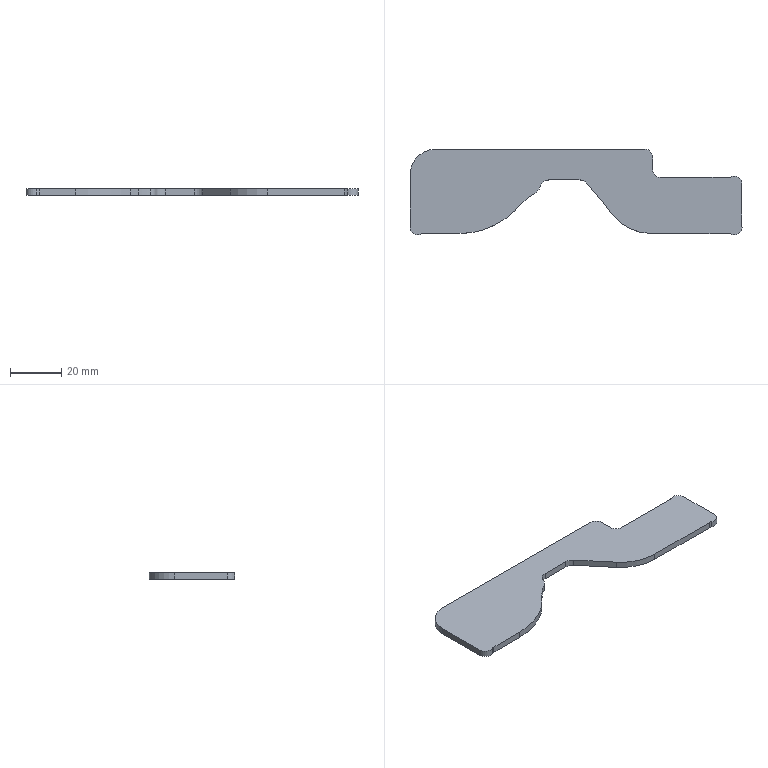Part | STEP file | lll_id342_x_t | 1 solid | 27 faces | box 130 x 33.5 x 2.5 mm | volume 7847 mm3 | cylinder 15 | plane 12 | commonest cylinder face diameters 6 x8 8 x3 20 x1 38 x1 39.772 x1 59.996 x1
STEP:
#1=CARTESIAN_POINT('',(708.5,-40.5,0.));
#2=VERTEX_POINT('',#1);
#3=CARTESIAN_POINT('',(708.5,-40.5,2.5));
#4=VERTEX_POINT('',#3);
#5=CARTESIAN_POINT('',(708.5,-40.5,-2.5));
#6=DIRECTION('',(0.,0.,1.));
#7=VECTOR('',#6,1.);
#8=LINE('',#5,#7);
#9=EDGE_CURVE('',#2,#4,#8,.T.);
#10=ORIENTED_EDGE('',*,*,#9,.T.);
#11=CARTESIAN_POINT('',(693.945,-33.713,2.5));
#12=VERTEX_POINT('',#11);
#13=CARTESIAN_POINT('',(708.5,-21.5,2.5));
#14=DIRECTION('',(0.,0.,-1.));
#15=DIRECTION('',(-1.,0.,0.));
#16=AXIS2_PLACEMENT_3D('',#13,#14,#15);
#17=CIRCLE('',#16,19.);
#18=EDGE_CURVE('',#4,#12,#17,.T.);
#19=ORIENTED_EDGE('',*,*,#18,.T.);
#20=CARTESIAN_POINT('',(693.945,-33.713,0.));
#21=VERTEX_POINT('',#20);
#22=CARTESIAN_POINT('',(693.945,-33.713,-2.5));
#23=DIRECTION('',(0.,0.,1.));
#24=VECTOR('',#23,1.);
#25=LINE('',#22,#24);
#26=EDGE_CURVE('',#21,#12,#25,.T.);
#27=ORIENTED_EDGE('',*,*,#26,.F.);
#28=CARTESIAN_POINT('',(708.5,-21.5,0.));
#29=DIRECTION('',(0.,0.,1.));
#30=DIRECTION('',(-1.,0.,0.));
#31=AXIS2_PLACEMENT_3D('',#28,#29,#30);
#32=CIRCLE('',#31,19.);
#33=EDGE_CURVE('',#21,#2,#32,.T.);
#34=ORIENTED_EDGE('',*,*,#33,.T.);
#35=EDGE_LOOP('',(#10,#19,#27,#34));
#36=FACE_OUTER_BOUND('',#35,.T.);
#37=CARTESIAN_POINT('',(708.5,-21.5,-2.5));
#38=DIRECTION('',(0.,0.,1.));
#39=DIRECTION('',(1.,0.,0.));
#40=AXIS2_PLACEMENT_3D('',#37,#38,#39);
#41=CYLINDRICAL_SURFACE('',#40,19.);
#42=ADVANCED_FACE('',(#36),#41,.T.);
#43=CARTESIAN_POINT('',(738.602,-40.5,0.));
#44=VERTEX_POINT('',#43);
#45=CARTESIAN_POINT('',(738.602,-40.5,2.5));
#46=VERTEX_POINT('',#45);
#47=CARTESIAN_POINT('',(738.602,-40.5,-2.5));
#48=DIRECTION('',(0.,0.,1.));
#49=VECTOR('',#48,1.);
#50=LINE('',#47,#49);
#51=EDGE_CURVE('',#44,#46,#50,.T.);
#52=ORIENTED_EDGE('',*,*,#51,.T.);
#53=CARTESIAN_POINT('',(12273.883,-40.5,2.5));
#54=DIRECTION('',(-1.,0.,0.));
#55=VECTOR('',#54,1.);
#56=LINE('',#53,#55);
#57=EDGE_CURVE('',#46,#4,#56,.T.);
#58=ORIENTED_EDGE('',*,*,#57,.T.);
#59=ORIENTED_EDGE('',*,*,#9,.F.);
#60=CARTESIAN_POINT('',(12283.883,-40.5,0.));
#61=DIRECTION('',(-1.,0.,0.));
#62=VECTOR('',#61,1.);
#63=LINE('',#60,#62);
#64=EDGE_CURVE('',#44,#2,#63,.T.);
#65=ORIENTED_EDGE('',*,*,#64,.F.);
#66=EDGE_LOOP('',(#52,#58,#59,#65));
#67=FACE_OUTER_BOUND('',#66,.T.);
#68=CARTESIAN_POINT('',(708.5,-40.5,-2.5));
#69=DIRECTION('',(0.,-1.,0.));
#70=DIRECTION('',(1.,0.,0.));
#71=AXIS2_PLACEMENT_3D('',#68,#69,#70);
#72=PLANE('',#71);
#73=ADVANCED_FACE('',(#67),#72,.T.);
#74=CARTESIAN_POINT('',(739.801,-40.75,0.));
#75=VERTEX_POINT('',#74);
#76=CARTESIAN_POINT('',(739.801,-40.75,2.5));
#77=VERTEX_POINT('',#76);
#78=CARTESIAN_POINT('',(739.801,-40.75,-2.5));
#79=DIRECTION('',(0.,0.,1.));
#80=VECTOR('',#79,1.);
#81=LINE('',#78,#80);
#82=EDGE_CURVE('',#75,#77,#81,.T.);
#83=ORIENTED_EDGE('',*,*,#82,.T.);
#84=CARTESIAN_POINT('',(738.602,-43.5,2.5));
#85=DIRECTION('',(0.,0.,1.));
#86=DIRECTION('',(-1.,0.,0.));
#87=AXIS2_PLACEMENT_3D('',#84,#85,#86);
#88=CIRCLE('',#87,3.);
#89=EDGE_CURVE('',#77,#46,#88,.T.);
#90=ORIENTED_EDGE('',*,*,#89,.T.);
#91=ORIENTED_EDGE('',*,*,#51,.F.);
#92=CARTESIAN_POINT('',(738.602,-43.5,0.));
#93=DIRECTION('',(0.,0.,-1.));
#94=DIRECTION('',(-1.,0.,0.));
#95=AXIS2_PLACEMENT_3D('',#92,#93,#94);
#96=CIRCLE('',#95,3.);
#97=EDGE_CURVE('',#44,#75,#96,.T.);
#98=ORIENTED_EDGE('',*,*,#97,.T.);
#99=EDGE_LOOP('',(#83,#90,#91,#98));
#100=FACE_OUTER_BOUND('',#99,.T.);
#101=CARTESIAN_POINT('',(738.602,-43.5,-2.5));
#102=DIRECTION('',(0.,0.,1.));
#103=DIRECTION('',(1.,0.,0.));
#104=AXIS2_PLACEMENT_3D('',#101,#102,#103);
#105=CYLINDRICAL_SURFACE('',#104,3.);
#106=ADVANCED_FACE('',(#100),#105,.F.);
#107=CARTESIAN_POINT('',(744.,-38.,0.));
#108=VERTEX_POINT('',#107);
#109=CARTESIAN_POINT('',(744.,-38.,2.5));
#110=VERTEX_POINT('',#109);
#111=CARTESIAN_POINT('',(744.,-38.,-2.5));
#112=DIRECTION('',(0.,0.,1.));
#113=VECTOR('',#112,1.);
#114=LINE('',#111,#113);
#115=EDGE_CURVE('',#108,#110,#114,.T.);
#116=ORIENTED_EDGE('',*,*,#115,.T.);
#117=CARTESIAN_POINT('',(741.,-38.,2.5));
#118=DIRECTION('',(0.,0.,-1.));
#119=DIRECTION('',(-1.,0.,0.));
#120=AXIS2_PLACEMENT_3D('',#117,#118,#119);
#121=CIRCLE('',#120,3.);
#122=EDGE_CURVE('',#110,#77,#121,.T.);
#123=ORIENTED_EDGE('',*,*,#122,.T.);
#124=ORIENTED_EDGE('',*,*,#82,.F.);
#125=CARTESIAN_POINT('',(741.,-38.,0.));
#126=DIRECTION('',(0.,0.,-1.));
#127=DIRECTION('',(-1.,0.,0.));
#128=AXIS2_PLACEMENT_3D('',#125,#126,#127);
#129=CIRCLE('',#128,3.);
#130=EDGE_CURVE('',#108,#75,#129,.T.);
#131=ORIENTED_EDGE('',*,*,#130,.F.);
#132=EDGE_LOOP('',(#116,#123,#124,#131));
#133=FACE_OUTER_BOUND('',#132,.T.);
#134=CARTESIAN_POINT('',(741.,-38.,-2.5));
#135=DIRECTION('',(0.,0.,1.));
#136=DIRECTION('',(1.,0.,0.));
#137=AXIS2_PLACEMENT_3D('',#134,#135,#136);
#138=CYLINDRICAL_SURFACE('',#137,3.);
#139=ADVANCED_FACE('',(#133),#138,.T.);
#140=ORIENTED_EDGE('',*,*,#26,.T.);
#141=CARTESIAN_POINT('',(683.218,-20.929,2.5));
#142=VERTEX_POINT('',#141);
#143=CARTESIAN_POINT('',(12214.125,-13762.929,2.5));
#144=DIRECTION('',(0.6428,-0.766,0.));
#145=VECTOR('',#144,1.);
#146=LINE('',#143,#145);
#147=EDGE_CURVE('',#142,#12,#146,.T.);
#148=ORIENTED_EDGE('',*,*,#147,.F.);
#149=CARTESIAN_POINT('',(683.218,-20.929,0.));
#150=VERTEX_POINT('',#149);
#151=CARTESIAN_POINT('',(683.218,-20.929,-2.5));
#152=DIRECTION('',(0.,0.,1.));
#153=VECTOR('',#152,1.);
#154=LINE('',#151,#153);
#155=EDGE_CURVE('',#150,#142,#154,.T.);
#156=ORIENTED_EDGE('',*,*,#155,.F.);
#157=CARTESIAN_POINT('',(12218.257,-13767.853,0.));
#158=DIRECTION('',(0.6428,-0.766,0.));
#159=VECTOR('',#158,1.);
#160=LINE('',#157,#159);
#161=EDGE_CURVE('',#150,#21,#160,.T.);
#162=ORIENTED_EDGE('',*,*,#161,.T.);
#163=EDGE_LOOP('',(#140,#148,#156,#162));
#164=FACE_OUTER_BOUND('',#163,.T.);
#165=CARTESIAN_POINT('',(683.218,-20.929,-2.5));
#166=DIRECTION('',(-0.766,-0.6428,0.));
#167=DIRECTION('',(0.6428,-0.766,0.));
#168=AXIS2_PLACEMENT_3D('',#165,#166,#167);
#169=PLANE('',#168);
#170=ADVANCED_FACE('',(#164),#169,.T.);
#171=CARTESIAN_POINT('',(744.,-21.,0.));
#172=VERTEX_POINT('',#171);
#173=CARTESIAN_POINT('',(744.,-13712.786,0.));
#174=DIRECTION('',(0.,-1.,0.));
#175=VECTOR('',#174,1.);
#176=LINE('',#173,#175);
#177=EDGE_CURVE('',#172,#108,#176,.T.);
#178=ORIENTED_EDGE('',*,*,#177,.F.);
#179=CARTESIAN_POINT('',(744.,-21.,2.5));
#180=VERTEX_POINT('',#179);
#181=CARTESIAN_POINT('',(744.,-21.,2.5));
#182=DIRECTION('',(0.,0.,-1.));
#183=VECTOR('',#182,1.);
#184=LINE('',#181,#183);
#185=EDGE_CURVE('',#180,#172,#184,.T.);
#186=ORIENTED_EDGE('',*,*,#185,.F.);
#187=CARTESIAN_POINT('',(744.,-13712.786,2.5));
#188=DIRECTION('',(0.,-1.,0.));
#189=VECTOR('',#188,1.);
#190=LINE('',#187,#189);
#191=EDGE_CURVE('',#180,#110,#190,.T.);
#192=ORIENTED_EDGE('',*,*,#191,.T.);
#193=ORIENTED_EDGE('',*,*,#115,.F.);
#194=EDGE_LOOP('',(#178,#186,#192,#193));
#195=FACE_OUTER_BOUND('',#194,.T.);
#196=CARTESIAN_POINT('',(744.,-38.,-2.5));
#197=DIRECTION('',(1.,0.,0.));
#198=DIRECTION('',(0.,1.,0.));
#199=AXIS2_PLACEMENT_3D('',#196,#197,#198);
#200=PLANE('',#199);
#201=ADVANCED_FACE('',(#195),#200,.T.);
#202=CARTESIAN_POINT('',(739.801,-18.25,0.));
#203=VERTEX_POINT('',#202);
#204=CARTESIAN_POINT('',(741.,-21.,0.));
#205=DIRECTION('',(0.,0.,1.));
#206=DIRECTION('',(-1.,0.,0.));
#207=AXIS2_PLACEMENT_3D('',#204,#205,#206);
#208=CIRCLE('',#207,3.);
#209=EDGE_CURVE('',#172,#203,#208,.T.);
#210=ORIENTED_EDGE('',*,*,#209,.F.);
#211=ORIENTED_EDGE('',*,*,#177,.T.);
#212=ORIENTED_EDGE('',*,*,#130,.T.);
#213=ORIENTED_EDGE('',*,*,#97,.F.);
#214=ORIENTED_EDGE('',*,*,#64,.T.);
#215=ORIENTED_EDGE('',*,*,#33,.F.);
#216=ORIENTED_EDGE('',*,*,#161,.F.);
#217=CARTESIAN_POINT('',(680.154,-19.5,0.));
#218=VERTEX_POINT('',#217);
#219=CARTESIAN_POINT('',(680.154,-23.5,0.));
#220=DIRECTION('',(0.,0.,1.));
#221=DIRECTION('',(1.,0.,0.));
#222=AXIS2_PLACEMENT_3D('',#219,#220,#221);
#223=CIRCLE('',#222,4.);
#224=EDGE_CURVE('',#150,#218,#223,.T.);
#225=ORIENTED_EDGE('',*,*,#224,.T.);
#226=CARTESIAN_POINT('',(668.697,-19.5,0.));
#227=VERTEX_POINT('',#226);
#228=CARTESIAN_POINT('',(665.5,-19.5,0.));
#229=DIRECTION('',(1.,0.,0.));
#230=VECTOR('',#229,1.);
#231=LINE('',#228,#230);
#232=EDGE_CURVE('',#227,#218,#231,.T.);
#233=ORIENTED_EDGE('',*,*,#232,.F.);
#234=CARTESIAN_POINT('',(664.848,-22.409,0.));
#235=VERTEX_POINT('',#234);
#236=CARTESIAN_POINT('',(668.697,-23.5,0.));
#237=DIRECTION('',(0.,0.,-1.));
#238=DIRECTION('',(-1.,0.,0.));
#239=AXIS2_PLACEMENT_3D('',#236,#237,#238);
#240=CIRCLE('',#239,4.);
#241=EDGE_CURVE('',#235,#227,#240,.T.);
#242=ORIENTED_EDGE('',*,*,#241,.F.);
#243=CARTESIAN_POINT('',(662.881,-24.849,0.));
#244=VERTEX_POINT('',#243);
#245=CARTESIAN_POINT('',(661.,-21.318,0.));
#246=DIRECTION('',(0.,0.,1.));
#247=DIRECTION('',(-1.,0.,0.));
#248=AXIS2_PLACEMENT_3D('',#245,#246,#247);
#249=CIRCLE('',#248,4.);
#250=EDGE_CURVE('',#244,#235,#249,.T.);
#251=ORIENTED_EDGE('',*,*,#250,.F.);
#252=CARTESIAN_POINT('',(658.142,-28.358,0.));
#253=VERTEX_POINT('',#252);
#254=CARTESIAN_POINT('',(672.216,-42.407,0.));
#255=DIRECTION('',(0.,0.,-1.));
#256=DIRECTION('',(-1.,0.,0.));
#257=AXIS2_PLACEMENT_3D('',#254,#255,#256);
#258=CIRCLE('',#257,19.886);
#259=EDGE_CURVE('',#253,#244,#258,.T.);
#260=ORIENTED_EDGE('',*,*,#259,.F.);
#261=CARTESIAN_POINT('',(654.787,-31.713,0.));
#262=VERTEX_POINT('',#261);
#263=CARTESIAN_POINT('',(654.787,-31.713,0.));
#264=DIRECTION('',(0.7071,0.7071,0.));
#265=VECTOR('',#264,1.);
#266=LINE('',#263,#265);
#267=EDGE_CURVE('',#262,#253,#266,.T.);
#268=ORIENTED_EDGE('',*,*,#267,.F.);
#269=CARTESIAN_POINT('',(633.574,-40.5,0.));
#270=VERTEX_POINT('',#269);
#271=CARTESIAN_POINT('',(633.574,-10.502,0.));
#272=DIRECTION('',(0.,0.,1.));
#273=DIRECTION('',(-1.,0.,0.));
#274=AXIS2_PLACEMENT_3D('',#271,#272,#273);
#275=CIRCLE('',#274,29.998);
#276=EDGE_CURVE('',#270,#262,#275,.T.);
#277=ORIENTED_EDGE('',*,*,#276,.F.);
#278=CARTESIAN_POINT('',(619.398,-40.5,0.));
#279=VERTEX_POINT('',#278);
#280=CARTESIAN_POINT('',(619.398,-40.5,0.));
#281=DIRECTION('',(1.,0.,0.));
#282=VECTOR('',#281,1.);
#283=LINE('',#280,#282);
#284=EDGE_CURVE('',#279,#270,#283,.T.);
#285=ORIENTED_EDGE('',*,*,#284,.F.);
#286=CARTESIAN_POINT('',(618.199,-40.75,0.));
#287=VERTEX_POINT('',#286);
#288=CARTESIAN_POINT('',(619.398,-43.5,0.));
#289=DIRECTION('',(0.,0.,-1.));
#290=DIRECTION('',(-1.,0.,0.));
#291=AXIS2_PLACEMENT_3D('',#288,#289,#290);
#292=CIRCLE('',#291,3.);
#293=EDGE_CURVE('',#287,#279,#292,.T.);
#294=ORIENTED_EDGE('',*,*,#293,.F.);
#295=CARTESIAN_POINT('',(614.,-38.,0.));
#296=VERTEX_POINT('',#295);
#297=CARTESIAN_POINT('',(617.,-38.,0.));
#298=DIRECTION('',(0.,0.,1.));
#299=DIRECTION('',(-1.,0.,0.));
#300=AXIS2_PLACEMENT_3D('',#297,#298,#299);
#301=CIRCLE('',#300,3.);
#302=EDGE_CURVE('',#296,#287,#301,.T.);
#303=ORIENTED_EDGE('',*,*,#302,.F.);
#304=CARTESIAN_POINT('',(614.,-17.5,0.));
#305=VERTEX_POINT('',#304);
#306=CARTESIAN_POINT('',(614.,-17.5,0.));
#307=DIRECTION('',(0.,-1.,0.));
#308=VECTOR('',#307,1.);
#309=LINE('',#306,#308);
#310=EDGE_CURVE('',#305,#296,#309,.T.);
#311=ORIENTED_EDGE('',*,*,#310,.F.);
#312=CARTESIAN_POINT('',(624.,-7.5,0.));
#313=VERTEX_POINT('',#312);
#314=CARTESIAN_POINT('',(624.,-17.5,0.));
#315=DIRECTION('',(0.,0.,1.));
#316=DIRECTION('',(-1.,0.,0.));
#317=AXIS2_PLACEMENT_3D('',#314,#315,#316);
#318=CIRCLE('',#317,10.);
#319=EDGE_CURVE('',#313,#305,#318,.T.);
#320=ORIENTED_EDGE('',*,*,#319,.F.);
#321=CARTESIAN_POINT('',(706.,-7.5,0.));
#322=VERTEX_POINT('',#321);
#323=CARTESIAN_POINT('',(706.,-7.5,0.));
#324=DIRECTION('',(-1.,0.,0.));
#325=VECTOR('',#324,1.);
#326=LINE('',#323,#325);
#327=EDGE_CURVE('',#322,#313,#326,.T.);
#328=ORIENTED_EDGE('',*,*,#327,.F.);
#329=CARTESIAN_POINT('',(709.,-10.5,0.));
#330=VERTEX_POINT('',#329);
#331=CARTESIAN_POINT('',(706.,-10.5,0.));
#332=DIRECTION('',(0.,0.,1.));
#333=DIRECTION('',(-1.,0.,0.));
#334=AXIS2_PLACEMENT_3D('',#331,#332,#333);
#335=CIRCLE('',#334,3.);
#336=EDGE_CURVE('',#330,#322,#335,.T.);
#337=ORIENTED_EDGE('',*,*,#336,.F.);
#338=CARTESIAN_POINT('',(709.,-15.5,0.));
#339=VERTEX_POINT('',#338);
#340=CARTESIAN_POINT('',(709.,-15.5,0.));
#341=DIRECTION('',(0.,1.,0.));
#342=VECTOR('',#341,1.);
#343=LINE('',#340,#342);
#344=EDGE_CURVE('',#339,#330,#343,.T.);
#345=ORIENTED_EDGE('',*,*,#344,.F.);
#346=CARTESIAN_POINT('',(712.,-18.5,0.));
#347=VERTEX_POINT('',#346);
#348=CARTESIAN_POINT('',(712.,-15.5,0.));
#349=DIRECTION('',(0.,0.,-1.));
#350=DIRECTION('',(-1.,0.,0.));
#351=AXIS2_PLACEMENT_3D('',#348,#349,#350);
#352=CIRCLE('',#351,3.);
#353=EDGE_CURVE('',#347,#339,#352,.T.);
#354=ORIENTED_EDGE('',*,*,#353,.F.);
#355=CARTESIAN_POINT('',(738.602,-18.5,0.));
#356=VERTEX_POINT('',#355);
#357=CARTESIAN_POINT('',(738.602,-18.5,0.));
#358=DIRECTION('',(-1.,0.,0.));
#359=VECTOR('',#358,1.);
#360=LINE('',#357,#359);
#361=EDGE_CURVE('',#356,#347,#360,.T.);
#362=ORIENTED_EDGE('',*,*,#361,.F.);
#363=CARTESIAN_POINT('',(738.602,-15.5,0.));
#364=DIRECTION('',(0.,0.,-1.));
#365=DIRECTION('',(-1.,0.,0.));
#366=AXIS2_PLACEMENT_3D('',#363,#364,#365);
#367=CIRCLE('',#366,3.);
#368=EDGE_CURVE('',#203,#356,#367,.T.);
#369=ORIENTED_EDGE('',*,*,#368,.F.);
#370=EDGE_LOOP('',(#210,#211,#212,#213,#214,#215,#216,#225,#233,#242,#251,#260,#268,#277,#285,#294,#303,#311,#320,#328,#337,#345,#354,#362,#369));
#371=FACE_OUTER_BOUND('',#370,.T.);
#372=CARTESIAN_POINT('',(12283.883,-13712.786,0.));
#373=DIRECTION('',(0.,0.,-1.));
#374=DIRECTION('',(-1.,0.,0.));
#375=AXIS2_PLACEMENT_3D('',#372,#373,#374);
#376=PLANE('',#375);
#377=ADVANCED_FACE('',(#371),#376,.T.);
#378=ORIENTED_EDGE('',*,*,#191,.F.);
#379=CARTESIAN_POINT('',(739.801,-18.25,2.5));
#380=VERTEX_POINT('',#379);
#381=CARTESIAN_POINT('',(741.,-21.,2.5));
#382=DIRECTION('',(0.,0.,1.));
#383=DIRECTION('',(-1.,0.,0.));
#384=AXIS2_PLACEMENT_3D('',#381,#382,#383);
#385=CIRCLE('',#384,3.);
#386=EDGE_CURVE('',#180,#380,#385,.T.);
#387=ORIENTED_EDGE('',*,*,#386,.T.);
#388=CARTESIAN_POINT('',(738.602,-18.5,2.5));
#389=VERTEX_POINT('',#388);
#390=CARTESIAN_POINT('',(738.602,-15.5,2.5));
#391=DIRECTION('',(0.,0.,-1.));
#392=DIRECTION('',(-1.,0.,0.));
#393=AXIS2_PLACEMENT_3D('',#390,#391,#392);
#394=CIRCLE('',#393,3.);
#395=EDGE_CURVE('',#380,#389,#394,.T.);
#396=ORIENTED_EDGE('',*,*,#395,.T.);
#397=CARTESIAN_POINT('',(712.,-18.5,2.5));
#398=VERTEX_POINT('',#397);
#399=CARTESIAN_POINT('',(738.602,-18.5,2.5));
#400=DIRECTION('',(-1.,0.,0.));
#401=VECTOR('',#400,1.);
#402=LINE('',#399,#401);
#403=EDGE_CURVE('',#389,#398,#402,.T.);
#404=ORIENTED_EDGE('',*,*,#403,.T.);
#405=CARTESIAN_POINT('',(709.,-15.5,2.5));
#406=VERTEX_POINT('',#405);
#407=CARTESIAN_POINT('',(712.,-15.5,2.5));
#408=DIRECTION('',(0.,0.,-1.));
#409=DIRECTION('',(-1.,0.,0.));
#410=AXIS2_PLACEMENT_3D('',#407,#408,#409);
#411=CIRCLE('',#410,3.);
#412=EDGE_CURVE('',#398,#406,#411,.T.);
#413=ORIENTED_EDGE('',*,*,#412,.T.);
#414=CARTESIAN_POINT('',(709.,-10.5,2.5));
#415=VERTEX_POINT('',#414);
#416=CARTESIAN_POINT('',(709.,-15.5,2.5));
#417=DIRECTION('',(0.,1.,0.));
#418=VECTOR('',#417,1.);
#419=LINE('',#416,#418);
#420=EDGE_CURVE('',#406,#415,#419,.T.);
#421=ORIENTED_EDGE('',*,*,#420,.T.);
#422=CARTESIAN_POINT('',(706.,-7.5,2.5));
#423=VERTEX_POINT('',#422);
#424=CARTESIAN_POINT('',(706.,-10.5,2.5));
#425=DIRECTION('',(0.,0.,1.));
#426=DIRECTION('',(-1.,0.,0.));
#427=AXIS2_PLACEMENT_3D('',#424,#425,#426);
#428=CIRCLE('',#427,3.);
#429=EDGE_CURVE('',#415,#423,#428,.T.);
#430=ORIENTED_EDGE('',*,*,#429,.T.);
#431=CARTESIAN_POINT('',(624.,-7.5,2.5));
#432=VERTEX_POINT('',#431);
#433=CARTESIAN_POINT('',(706.,-7.5,2.5));
#434=DIRECTION('',(-1.,0.,0.));
#435=VECTOR('',#434,1.);
#436=LINE('',#433,#435);
#437=EDGE_CURVE('',#423,#432,#436,.T.);
#438=ORIENTED_EDGE('',*,*,#437,.T.);
#439=CARTESIAN_POINT('',(614.,-17.5,2.5));
#440=VERTEX_POINT('',#439);
#441=CARTESIAN_POINT('',(624.,-17.5,2.5));
#442=DIRECTION('',(0.,0.,1.));
#443=DIRECTION('',(-1.,0.,0.));
#444=AXIS2_PLACEMENT_3D('',#441,#442,#443);
#445=CIRCLE('',#444,10.);
#446=EDGE_CURVE('',#432,#440,#445,.T.);
#447=ORIENTED_EDGE('',*,*,#446,.T.);
#448=CARTESIAN_POINT('',(614.,-38.,2.5));
#449=VERTEX_POINT('',#448);
#450=CARTESIAN_POINT('',(614.,-17.5,2.5));
#451=DIRECTION('',(0.,-1.,0.));
#452=VECTOR('',#451,1.);
#453=LINE('',#450,#452);
#454=EDGE_CURVE('',#440,#449,#453,.T.);
#455=ORIENTED_EDGE('',*,*,#454,.T.);
#456=CARTESIAN_POINT('',(618.199,-40.75,2.5));
#457=VERTEX_POINT('',#456);
#458=CARTESIAN_POINT('',(617.,-38.,2.5));
#459=DIRECTION('',(0.,0.,1.));
#460=DIRECTION('',(-1.,0.,0.));
#461=AXIS2_PLACEMENT_3D('',#458,#459,#460);
#462=CIRCLE('',#461,3.);
#463=EDGE_CURVE('',#449,#457,#462,.T.);
#464=ORIENTED_EDGE('',*,*,#463,.T.);
#465=CARTESIAN_POINT('',(619.398,-40.5,2.5));
#466=VERTEX_POINT('',#465);
#467=CARTESIAN_POINT('',(619.398,-43.5,2.5));
#468=DIRECTION('',(0.,0.,-1.));
#469=DIRECTION('',(-1.,0.,0.));
#470=AXIS2_PLACEMENT_3D('',#467,#468,#469);
#471=CIRCLE('',#470,3.);
#472=EDGE_CURVE('',#457,#466,#471,.T.);
#473=ORIENTED_EDGE('',*,*,#472,.T.);
#474=CARTESIAN_POINT('',(633.574,-40.5,2.5));
#475=VERTEX_POINT('',#474);
#476=CARTESIAN_POINT('',(619.398,-40.5,2.5));
#477=DIRECTION('',(1.,0.,0.));
#478=VECTOR('',#477,1.);
#479=LINE('',#476,#478);
#480=EDGE_CURVE('',#466,#475,#479,.T.);
#481=ORIENTED_EDGE('',*,*,#480,.T.);
#482=CARTESIAN_POINT('',(654.787,-31.713,2.5));
#483=VERTEX_POINT('',#482);
#484=CARTESIAN_POINT('',(633.574,-10.502,2.5));
#485=DIRECTION('',(0.,0.,1.));
#486=DIRECTION('',(-1.,0.,0.));
#487=AXIS2_PLACEMENT_3D('',#484,#485,#486);
#488=CIRCLE('',#487,29.998);
#489=EDGE_CURVE('',#475,#483,#488,.T.);
#490=ORIENTED_EDGE('',*,*,#489,.T.);
#491=CARTESIAN_POINT('',(658.142,-28.358,2.5));
#492=VERTEX_POINT('',#491);
#493=CARTESIAN_POINT('',(654.787,-31.713,2.5));
#494=DIRECTION('',(0.7071,0.7071,0.));
#495=VECTOR('',#494,1.);
#496=LINE('',#493,#495);
#497=EDGE_CURVE('',#483,#492,#496,.T.);
#498=ORIENTED_EDGE('',*,*,#497,.T.);
#499=CARTESIAN_POINT('',(662.881,-24.849,2.5));
#500=VERTEX_POINT('',#499);
#501=CARTESIAN_POINT('',(672.216,-42.407,2.5));
#502=DIRECTION('',(0.,0.,-1.));
#503=DIRECTION('',(-1.,0.,0.));
#504=AXIS2_PLACEMENT_3D('',#501,#502,#503);
#505=CIRCLE('',#504,19.886);
#506=EDGE_CURVE('',#492,#500,#505,.T.);
#507=ORIENTED_EDGE('',*,*,#506,.T.);
#508=CARTESIAN_POINT('',(664.848,-22.409,2.5));
#509=VERTEX_POINT('',#508);
#510=CARTESIAN_POINT('',(661.,-21.318,2.5));
#511=DIRECTION('',(0.,0.,1.));
#512=DIRECTION('',(-1.,0.,0.));
#513=AXIS2_PLACEMENT_3D('',#510,#511,#512);
#514=CIRCLE('',#513,4.);
#515=EDGE_CURVE('',#500,#509,#514,.T.);
#516=ORIENTED_EDGE('',*,*,#515,.T.);
#517=CARTESIAN_POINT('',(668.697,-19.5,2.5));
#518=VERTEX_POINT('',#517);
#519=CARTESIAN_POINT('',(668.697,-23.5,2.5));
#520=DIRECTION('',(0.,0.,1.));
#521=DIRECTION('',(-1.,0.,0.));
#522=AXIS2_PLACEMENT_3D('',#519,#520,#521);
#523=CIRCLE('',#522,4.);
#524=EDGE_CURVE('',#518,#509,#523,.T.);
#525=ORIENTED_EDGE('',*,*,#524,.F.);
#526=CARTESIAN_POINT('',(680.154,-19.5,2.5));
#527=VERTEX_POINT('',#526);
#528=CARTESIAN_POINT('',(665.5,-19.5,2.5));
#529=DIRECTION('',(1.,0.,0.));
#530=VECTOR('',#529,1.);
#531=LINE('',#528,#530);
#532=EDGE_CURVE('',#518,#527,#531,.T.);
#533=ORIENTED_EDGE('',*,*,#532,.T.);
#534=CARTESIAN_POINT('',(680.154,-23.5,2.5));
#535=DIRECTION('',(0.,0.,-1.));
#536=DIRECTION('',(1.,0.,0.));
#537=AXIS2_PLACEMENT_3D('',#534,#535,#536);
#538=CIRCLE('',#537,4.);
#539=EDGE_CURVE('',#527,#142,#538,.T.);
#540=ORIENTED_EDGE('',*,*,#539,.T.);
#541=ORIENTED_EDGE('',*,*,#147,.T.);
#542=ORIENTED_EDGE('',*,*,#18,.F.);
#543=ORIENTED_EDGE('',*,*,#57,.F.);
#544=ORIENTED_EDGE('',*,*,#89,.F.);
#545=ORIENTED_EDGE('',*,*,#122,.F.);
#546=EDGE_LOOP('',(#378,#387,#396,#404,#413,#421,#430,#438,#447,#455,#464,#473,#481,#490,#498,#507,#516,#525,#533,#540,#541,#542,#543,#544,#545));
#547=FACE_OUTER_BOUND('',#546,.T.);
#548=CARTESIAN_POINT('',(12273.883,-13712.786,2.5));
#549=DIRECTION('',(0.,0.,-1.));
#550=DIRECTION('',(-1.,0.,0.));
#551=AXIS2_PLACEMENT_3D('',#548,#549,#550);
#552=PLANE('',#551);
#553=ADVANCED_FACE('',(#547),#552,.F.);
#554=ORIENTED_EDGE('',*,*,#250,.T.);
#555=CARTESIAN_POINT('',(664.848,-22.409,-2.5));
#556=DIRECTION('',(0.,0.,-1.));
#557=VECTOR('',#556,1.);
#558=LINE('',#555,#557);
#559=EDGE_CURVE('',#509,#235,#558,.T.);
#560=ORIENTED_EDGE('',*,*,#559,.F.);
#561=ORIENTED_EDGE('',*,*,#515,.F.);
#562=CARTESIAN_POINT('',(662.881,-24.849,2.5));
#563=DIRECTION('',(0.,0.,-1.));
#564=VECTOR('',#563,1.);
#565=LINE('',#562,#564);
#566=EDGE_CURVE('',#500,#244,#565,.T.);
#567=ORIENTED_EDGE('',*,*,#566,.T.);
#568=EDGE_LOOP('',(#554,#560,#561,#567));
#569=FACE_OUTER_BOUND('',#568,.T.);
#570=CARTESIAN_POINT('',(661.,-21.318,2.5));
#571=DIRECTION('',(0.,0.,-1.));
#572=DIRECTION('',(-1.,0.,0.));
#573=AXIS2_PLACEMENT_3D('',#570,#571,#572);
#574=CYLINDRICAL_SURFACE('',#573,4.);
#575=ADVANCED_FACE('',(#569),#574,.T.);
#576=CARTESIAN_POINT('',(668.697,-19.5,-2.5));
#577=DIRECTION('',(0.,0.,1.));
#578=VECTOR('',#577,1.);
#579=LINE('',#576,#578);
#580=EDGE_CURVE('',#227,#518,#579,.T.);
#581=ORIENTED_EDGE('',*,*,#580,.F.);
#582=ORIENTED_EDGE('',*,*,#232,.T.);
#583=CARTESIAN_POINT('',(680.154,-19.5,-2.5));
#584=DIRECTION('',(0.,0.,1.));
#585=VECTOR('',#584,1.);
#586=LINE('',#583,#585);
#587=EDGE_CURVE('',#218,#527,#586,.T.);
#588=ORIENTED_EDGE('',*,*,#587,.T.);
#589=ORIENTED_EDGE('',*,*,#532,.F.);
#590=EDGE_LOOP('',(#581,#582,#588,#589));
#591=FACE_OUTER_BOUND('',#590,.T.);
#592=CARTESIAN_POINT('',(665.5,-19.5,2.5));
#593=DIRECTION('',(0.,1.,0.));
#594=DIRECTION('',(0.,0.,1.));
#595=AXIS2_PLACEMENT_3D('',#592,#593,#594);
#596=PLANE('',#595);
#597=ADVANCED_FACE('',(#591),#596,.F.);
#598=ORIENTED_EDGE('',*,*,#209,.T.);
#599=CARTESIAN_POINT('',(739.801,-18.25,2.5));
#600=DIRECTION('',(0.,0.,-1.));
#601=VECTOR('',#600,1.);
#602=LINE('',#599,#601);
#603=EDGE_CURVE('',#380,#203,#602,.T.);
#604=ORIENTED_EDGE('',*,*,#603,.F.);
#605=ORIENTED_EDGE('',*,*,#386,.F.);
#606=ORIENTED_EDGE('',*,*,#185,.T.);
#607=EDGE_LOOP('',(#598,#604,#605,#606));
#608=FACE_OUTER_BOUND('',#607,.T.);
#609=CARTESIAN_POINT('',(741.,-21.,2.5));
#610=DIRECTION('',(0.,0.,-1.));
#611=DIRECTION('',(-1.,0.,0.));
#612=AXIS2_PLACEMENT_3D('',#609,#610,#611);
#613=CYLINDRICAL_SURFACE('',#612,3.);
#614=ADVANCED_FACE('',(#608),#613,.T.);
#615=ORIENTED_EDGE('',*,*,#368,.T.);
#616=CARTESIAN_POINT('',(738.602,-18.5,2.5));
#617=DIRECTION('',(0.,0.,-1.));
#618=VECTOR('',#617,1.);
#619=LINE('',#616,#618);
#620=EDGE_CURVE('',#389,#356,#619,.T.);
#621=ORIENTED_EDGE('',*,*,#620,.F.);
#622=ORIENTED_EDGE('',*,*,#395,.F.);
#623=ORIENTED_EDGE('',*,*,#603,.T.);
#624=EDGE_LOOP('',(#615,#621,#622,#623));
#625=FACE_OUTER_BOUND('',#624,.T.);
#626=CARTESIAN_POINT('',(738.602,-15.5,2.5));
#627=DIRECTION('',(0.,0.,-1.));
#628=DIRECTION('',(-1.,0.,0.));
#629=AXIS2_PLACEMENT_3D('',#626,#627,#628);
#630=CYLINDRICAL_SURFACE('',#629,3.);
#631=ADVANCED_FACE('',(#625),#630,.F.);
#632=ORIENTED_EDGE('',*,*,#361,.T.);
#633=CARTESIAN_POINT('',(712.,-18.5,2.5));
#634=DIRECTION('',(0.,0.,-1.));
#635=VECTOR('',#634,1.);
#636=LINE('',#633,#635);
#637=EDGE_CURVE('',#398,#347,#636,.T.);
#638=ORIENTED_EDGE('',*,*,#637,.F.);
#639=ORIENTED_EDGE('',*,*,#403,.F.);
#640=ORIENTED_EDGE('',*,*,#620,.T.);
#641=EDGE_LOOP('',(#632,#638,#639,#640));
#642=FACE_OUTER_BOUND('',#641,.T.);
#643=CARTESIAN_POINT('',(738.602,-18.5,2.5));
#644=DIRECTION('',(0.,-1.,0.));
#645=DIRECTION('',(0.,0.,-1.));
#646=AXIS2_PLACEMENT_3D('',#643,#644,#645);
#647=PLANE('',#646);
#648=ADVANCED_FACE('',(#642),#647,.F.);
#649=ORIENTED_EDGE('',*,*,#353,.T.);
#650=CARTESIAN_POINT('',(709.,-15.5,2.5));
#651=DIRECTION('',(0.,0.,-1.));
#652=VECTOR('',#651,1.);
#653=LINE('',#650,#652);
#654=EDGE_CURVE('',#406,#339,#653,.T.);
#655=ORIENTED_EDGE('',*,*,#654,.F.);
#656=ORIENTED_EDGE('',*,*,#412,.F.);
#657=ORIENTED_EDGE('',*,*,#637,.T.);
#658=EDGE_LOOP('',(#649,#655,#656,#657));
#659=FACE_OUTER_BOUND('',#658,.T.);
#660=CARTESIAN_POINT('',(712.,-15.5,2.5));
#661=DIRECTION('',(0.,0.,-1.));
#662=DIRECTION('',(-1.,0.,0.));
#663=AXIS2_PLACEMENT_3D('',#660,#661,#662);
#664=CYLINDRICAL_SURFACE('',#663,3.);
#665=ADVANCED_FACE('',(#659),#664,.F.);
#666=ORIENTED_EDGE('',*,*,#344,.T.);
#667=CARTESIAN_POINT('',(709.,-10.5,2.5));
#668=DIRECTION('',(0.,0.,-1.));
#669=VECTOR('',#668,1.);
#670=LINE('',#667,#669);
#671=EDGE_CURVE('',#415,#330,#670,.T.);
#672=ORIENTED_EDGE('',*,*,#671,.F.);
#673=ORIENTED_EDGE('',*,*,#420,.F.);
#674=ORIENTED_EDGE('',*,*,#654,.T.);
#675=EDGE_LOOP('',(#666,#672,#673,#674));
#676=FACE_OUTER_BOUND('',#675,.T.);
#677=CARTESIAN_POINT('',(709.,-15.5,2.5));
#678=DIRECTION('',(-1.,0.,0.));
#679=DIRECTION('',(0.,0.,1.));
#680=AXIS2_PLACEMENT_3D('',#677,#678,#679);
#681=PLANE('',#680);
#682=ADVANCED_FACE('',(#676),#681,.F.);
#683=ORIENTED_EDGE('',*,*,#336,.T.);
#684=CARTESIAN_POINT('',(706.,-7.5,2.5));
#685=DIRECTION('',(0.,0.,-1.));
#686=VECTOR('',#685,1.);
#687=LINE('',#684,#686);
#688=EDGE_CURVE('',#423,#322,#687,.T.);
#689=ORIENTED_EDGE('',*,*,#688,.F.);
#690=ORIENTED_EDGE('',*,*,#429,.F.);
#691=ORIENTED_EDGE('',*,*,#671,.T.);
#692=EDGE_LOOP('',(#683,#689,#690,#691));
#693=FACE_OUTER_BOUND('',#692,.T.);
#694=CARTESIAN_POINT('',(706.,-10.5,2.5));
#695=DIRECTION('',(0.,0.,-1.));
#696=DIRECTION('',(-1.,0.,0.));
#697=AXIS2_PLACEMENT_3D('',#694,#695,#696);
#698=CYLINDRICAL_SURFACE('',#697,3.);
#699=ADVANCED_FACE('',(#693),#698,.T.);
#700=ORIENTED_EDGE('',*,*,#327,.T.);
#701=CARTESIAN_POINT('',(624.,-7.5,2.5));
#702=DIRECTION('',(0.,0.,-1.));
#703=VECTOR('',#702,1.);
#704=LINE('',#701,#703);
#705=EDGE_CURVE('',#432,#313,#704,.T.);
#706=ORIENTED_EDGE('',*,*,#705,.F.);
#707=ORIENTED_EDGE('',*,*,#437,.F.);
#708=ORIENTED_EDGE('',*,*,#688,.T.);
#709=EDGE_LOOP('',(#700,#706,#707,#708));
#710=FACE_OUTER_BOUND('',#709,.T.);
#711=CARTESIAN_POINT('',(706.,-7.5,2.5));
#712=DIRECTION('',(0.,-1.,0.));
#713=DIRECTION('',(0.,0.,-1.));
#714=AXIS2_PLACEMENT_3D('',#711,#712,#713);
#715=PLANE('',#714);
#716=ADVANCED_FACE('',(#710),#715,.F.);
#717=ORIENTED_EDGE('',*,*,#319,.T.);
#718=CARTESIAN_POINT('',(614.,-17.5,2.5));
#719=DIRECTION('',(0.,0.,-1.));
#720=VECTOR('',#719,1.);
#721=LINE('',#718,#720);
#722=EDGE_CURVE('',#440,#305,#721,.T.);
#723=ORIENTED_EDGE('',*,*,#722,.F.);
#724=ORIENTED_EDGE('',*,*,#446,.F.);
#725=ORIENTED_EDGE('',*,*,#705,.T.);
#726=EDGE_LOOP('',(#717,#723,#724,#725));
#727=FACE_OUTER_BOUND('',#726,.T.);
#728=CARTESIAN_POINT('',(624.,-17.5,2.5));
#729=DIRECTION('',(0.,0.,-1.));
#730=DIRECTION('',(-1.,0.,0.));
#731=AXIS2_PLACEMENT_3D('',#728,#729,#730);
#732=CYLINDRICAL_SURFACE('',#731,10.);
#733=ADVANCED_FACE('',(#727),#732,.T.);
#734=ORIENTED_EDGE('',*,*,#310,.T.);
#735=CARTESIAN_POINT('',(614.,-38.,2.5));
#736=DIRECTION('',(0.,0.,-1.));
#737=VECTOR('',#736,1.);
#738=LINE('',#735,#737);
#739=EDGE_CURVE('',#449,#296,#738,.T.);
#740=ORIENTED_EDGE('',*,*,#739,.F.);
#741=ORIENTED_EDGE('',*,*,#454,.F.);
#742=ORIENTED_EDGE('',*,*,#722,.T.);
#743=EDGE_LOOP('',(#734,#740,#741,#742));
#744=FACE_OUTER_BOUND('',#743,.T.);
#745=CARTESIAN_POINT('',(614.,-17.5,2.5));
#746=DIRECTION('',(1.,0.,0.));
#747=DIRECTION('',(0.,0.,-1.));
#748=AXIS2_PLACEMENT_3D('',#745,#746,#747);
#749=PLANE('',#748);
#750=ADVANCED_FACE('',(#744),#749,.F.);
#751=ORIENTED_EDGE('',*,*,#302,.T.);
#752=CARTESIAN_POINT('',(618.199,-40.75,2.5));
#753=DIRECTION('',(0.,0.,-1.));
#754=VECTOR('',#753,1.);
#755=LINE('',#752,#754);
#756=EDGE_CURVE('',#457,#287,#755,.T.);
#757=ORIENTED_EDGE('',*,*,#756,.F.);
#758=ORIENTED_EDGE('',*,*,#463,.F.);
#759=ORIENTED_EDGE('',*,*,#739,.T.);
#760=EDGE_LOOP('',(#751,#757,#758,#759));
#761=FACE_OUTER_BOUND('',#760,.T.);
#762=CARTESIAN_POINT('',(617.,-38.,2.5));
#763=DIRECTION('',(0.,0.,-1.));
#764=DIRECTION('',(-1.,0.,0.));
#765=AXIS2_PLACEMENT_3D('',#762,#763,#764);
#766=CYLINDRICAL_SURFACE('',#765,3.);
#767=ADVANCED_FACE('',(#761),#766,.T.);
#768=ORIENTED_EDGE('',*,*,#293,.T.);
#769=CARTESIAN_POINT('',(619.398,-40.5,2.5));
#770=DIRECTION('',(0.,0.,-1.));
#771=VECTOR('',#770,1.);
#772=LINE('',#769,#771);
#773=EDGE_CURVE('',#466,#279,#772,.T.);
#774=ORIENTED_EDGE('',*,*,#773,.F.);
#775=ORIENTED_EDGE('',*,*,#472,.F.);
#776=ORIENTED_EDGE('',*,*,#756,.T.);
#777=EDGE_LOOP('',(#768,#774,#775,#776));
#778=FACE_OUTER_BOUND('',#777,.T.);
#779=CARTESIAN_POINT('',(619.398,-43.5,2.5));
#780=DIRECTION('',(0.,0.,-1.));
#781=DIRECTION('',(-1.,0.,0.));
#782=AXIS2_PLACEMENT_3D('',#779,#780,#781);
#783=CYLINDRICAL_SURFACE('',#782,3.);
#784=ADVANCED_FACE('',(#778),#783,.F.);
#785=ORIENTED_EDGE('',*,*,#284,.T.);
#786=CARTESIAN_POINT('',(633.574,-40.5,2.5));
#787=DIRECTION('',(0.,0.,-1.));
#788=VECTOR('',#787,1.);
#789=LINE('',#786,#788);
#790=EDGE_CURVE('',#475,#270,#789,.T.);
#791=ORIENTED_EDGE('',*,*,#790,.F.);
#792=ORIENTED_EDGE('',*,*,#480,.F.);
#793=ORIENTED_EDGE('',*,*,#773,.T.);
#794=EDGE_LOOP('',(#785,#791,#792,#793));
#795=FACE_OUTER_BOUND('',#794,.T.);
#796=CARTESIAN_POINT('',(619.398,-40.5,2.5));
#797=DIRECTION('',(0.,1.,0.));
#798=DIRECTION('',(0.,0.,1.));
#799=AXIS2_PLACEMENT_3D('',#796,#797,#798);
#800=PLANE('',#799);
#801=ADVANCED_FACE('',(#795),#800,.F.);
#802=ORIENTED_EDGE('',*,*,#276,.T.);
#803=CARTESIAN_POINT('',(654.787,-31.713,2.5));
#804=DIRECTION('',(0.,0.,-1.));
#805=VECTOR('',#804,1.);
#806=LINE('',#803,#805);
#807=EDGE_CURVE('',#483,#262,#806,.T.);
#808=ORIENTED_EDGE('',*,*,#807,.F.);
#809=ORIENTED_EDGE('',*,*,#489,.F.);
#810=ORIENTED_EDGE('',*,*,#790,.T.);
#811=EDGE_LOOP('',(#802,#808,#809,#810));
#812=FACE_OUTER_BOUND('',#811,.T.);
#813=CARTESIAN_POINT('',(633.574,-10.502,2.5));
#814=DIRECTION('',(0.,0.,-1.));
#815=DIRECTION('',(-1.,0.,0.));
#816=AXIS2_PLACEMENT_3D('',#813,#814,#815);
#817=CYLINDRICAL_SURFACE('',#816,29.998);
#818=ADVANCED_FACE('',(#812),#817,.T.);
#819=ORIENTED_EDGE('',*,*,#267,.T.);
#820=CARTESIAN_POINT('',(658.142,-28.358,2.5));
#821=DIRECTION('',(0.,0.,-1.));
#822=VECTOR('',#821,1.);
#823=LINE('',#820,#822);
#824=EDGE_CURVE('',#492,#253,#823,.T.);
#825=ORIENTED_EDGE('',*,*,#824,.F.);
#826=ORIENTED_EDGE('',*,*,#497,.F.);
#827=ORIENTED_EDGE('',*,*,#807,.T.);
#828=EDGE_LOOP('',(#819,#825,#826,#827));
#829=FACE_OUTER_BOUND('',#828,.T.);
#830=CARTESIAN_POINT('',(654.787,-31.713,2.5));
#831=DIRECTION('',(-0.7071,0.7071,0.));
#832=DIRECTION('',(0.7071,0.7071,0.));
#833=AXIS2_PLACEMENT_3D('',#830,#831,#832);
#834=PLANE('',#833);
#835=ADVANCED_FACE('',(#829),#834,.F.);
#836=ORIENTED_EDGE('',*,*,#259,.T.);
#837=ORIENTED_EDGE('',*,*,#566,.F.);
#838=ORIENTED_EDGE('',*,*,#506,.F.);
#839=ORIENTED_EDGE('',*,*,#824,.T.);
#840=EDGE_LOOP('',(#836,#837,#838,#839));
#841=FACE_OUTER_BOUND('',#840,.T.);
#842=CARTESIAN_POINT('',(672.216,-42.407,2.5));
#843=DIRECTION('',(0.,0.,-1.));
#844=DIRECTION('',(-1.,0.,0.));
#845=AXIS2_PLACEMENT_3D('',#842,#843,#844);
#846=CYLINDRICAL_SURFACE('',#845,19.886);
#847=ADVANCED_FACE('',(#841),#846,.F.);
#848=ORIENTED_EDGE('',*,*,#539,.F.);
#849=ORIENTED_EDGE('',*,*,#587,.F.);
#850=ORIENTED_EDGE('',*,*,#224,.F.);
#851=ORIENTED_EDGE('',*,*,#155,.T.);
#852=EDGE_LOOP('',(#848,#849,#850,#851));
#853=FACE_OUTER_BOUND('',#852,.T.);
#854=CARTESIAN_POINT('',(680.154,-23.5,-2.5));
#855=DIRECTION('',(0.,0.,1.));
#856=DIRECTION('',(1.,0.,0.));
#857=AXIS2_PLACEMENT_3D('',#854,#855,#856);
#858=CYLINDRICAL_SURFACE('',#857,4.);
#859=ADVANCED_FACE('',(#853),#858,.F.);
#860=ORIENTED_EDGE('',*,*,#580,.T.);
#861=ORIENTED_EDGE('',*,*,#524,.T.);
#862=ORIENTED_EDGE('',*,*,#559,.T.);
#863=ORIENTED_EDGE('',*,*,#241,.T.);
#864=EDGE_LOOP('',(#860,#861,#862,#863));
#865=FACE_OUTER_BOUND('',#864,.T.);
#866=CARTESIAN_POINT('',(668.697,-23.5,-2.5));
#867=DIRECTION('',(0.,0.,1.));
#868=DIRECTION('',(1.,0.,0.));
#869=AXIS2_PLACEMENT_3D('',#866,#867,#868);
#870=CYLINDRICAL_SURFACE('',#869,4.);
#871=ADVANCED_FACE('',(#865),#870,.F.);
#872=CLOSED_SHELL('',(#42,#73,#106,#139,#170,#201,#377,#553,#575,#597,#614,#631,#648,#665,#682,#699,#716,#733,#750,#767,#784,#801,#818,#835,#847,#859,#871));
#873=MANIFOLD_SOLID_BREP('',#872);
#874=(LENGTH_UNIT()NAMED_UNIT(*)SI_UNIT(.MILLI.,.METRE.));
#875=UNCERTAINTY_MEASURE_WITH_UNIT(LENGTH_MEASURE(0.00002),#874,'','');
#876=(NAMED_UNIT(*)PLANE_ANGLE_UNIT()SI_UNIT($,.RADIAN.));
#877=PLANE_ANGLE_MEASURE_WITH_UNIT(PLANE_ANGLE_MEASURE(0.01745),#876);
#878=DIMENSIONAL_EXPONENTS(0.,0.,0.,0.,0.,0.,0.);
#879=(CONVERSION_BASED_UNIT('DEGREE',#877)NAMED_UNIT(#878)PLANE_ANGLE_UNIT());
#880=(NAMED_UNIT(*)SI_UNIT($,.STERADIAN.)SOLID_ANGLE_UNIT());
#881=(GEOMETRIC_REPRESENTATION_CONTEXT(3)GLOBAL_UNCERTAINTY_ASSIGNED_CONTEXT((#875))GLOBAL_UNIT_ASSIGNED_CONTEXT((#874,#879,#880))REPRESENTATION_CONTEXT('',''));
#882=ADVANCED_BREP_SHAPE_REPRESENTATION('',(#873),#881);